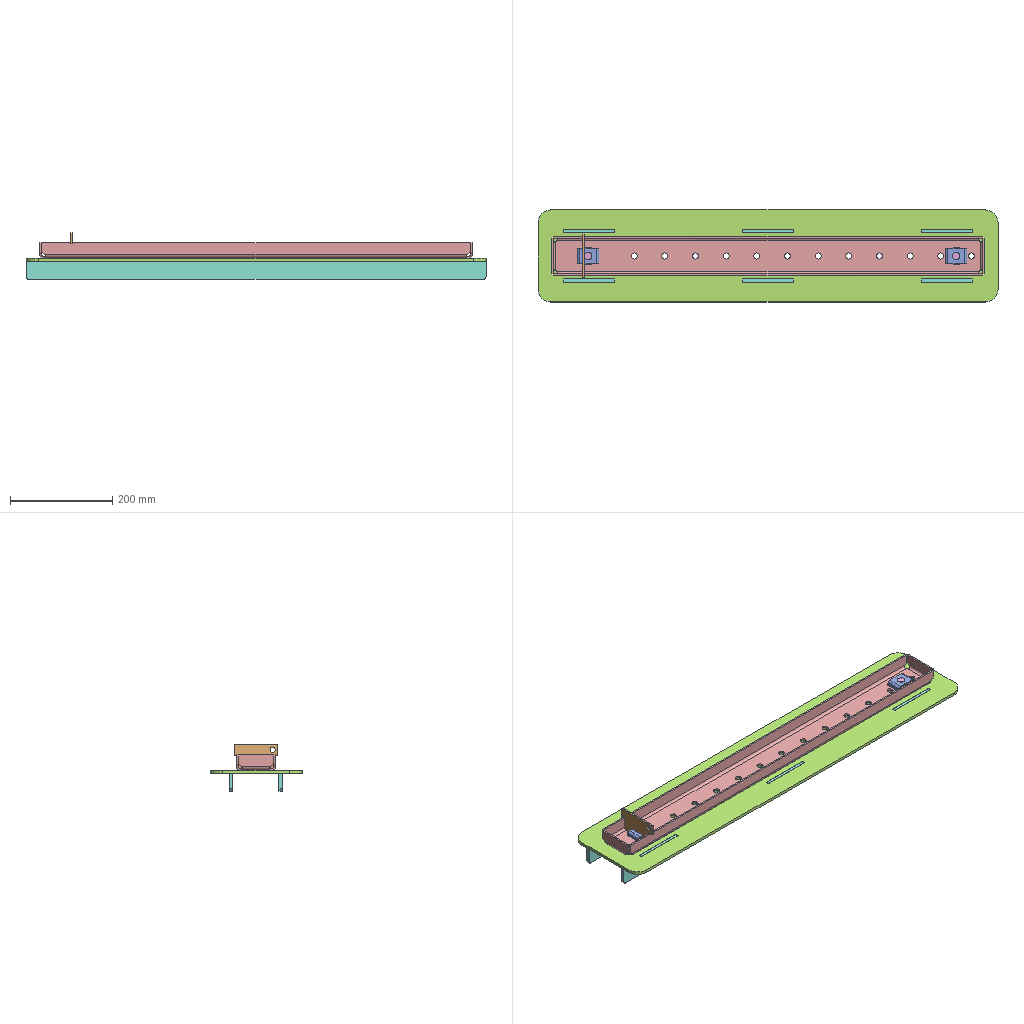Assembly | SolidWorks | 6 different items | 9 placed | box 900 x 180 x 91 mm
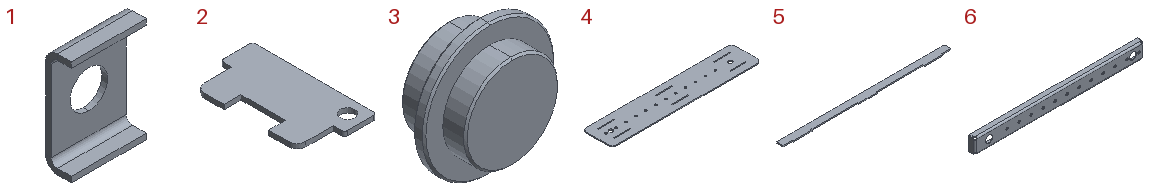Parts list (item | quantity | size | volume | features):
1 | x2 | 30 x 10.3 x 42 mm | 3379 mm3 | features FlatPattern 1, ICE 1, SMBaseFlange 1, SheetMetal 1
2 | x1 | 46.8 x 85 x 3.2 mm | 10065 mm3 | features FlatPattern 1, SMBaseFlange 1, SheetMetal 1
3 | x2 | 35 x 19.5 x 35 mm | 10211 mm3 | features Chamfer 1, Revolution 1
4 | x1 | 900 x 180 x 6 mm | 933147 mm3 | features FlatPattern 1, SMBaseFlange 1, SheetMetal 1
5 | x2 | 900 x 40.5 x 6 mm | 198836 mm3 | features FlatPattern 1, SMBaseFlange 1, SheetMetal 1
6 | x1 | 846 x 30 x 76.5 mm | 333721 mm3 | features ICE 2, CornerRelief 1, EdgeFlange 1, FlatPattern 1, LPattern 1, SMBaseFlange 1, SheetMetal 1
Mates (type | each side: item.copy, entity, surface, feature):
Coincident | 6.1 face plane Base-Flange1 | 1.1 face plane Base-Flange1
Concentric | 6.1 face cylinder Cut-Extrude2 | 1.1 face cylinder Cut-Extrude1
Parallel | 6.1 face plane Edge-Flange1 | 1.1 face plane Base-Flange1
InPlace | 6.1 face plane Base-Flange1 | 4.1 plane
InPlace | 6.1 plane | 3.1 plane
InPlace | 5.1 plane | assembly plane
InPlace | 2.1 plane | assembly plane